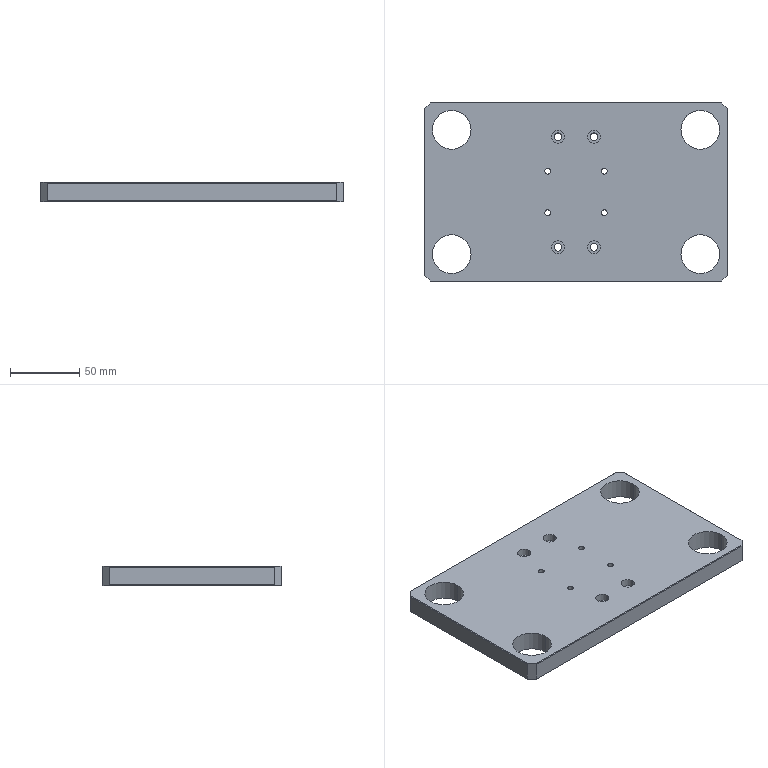Part | STEP file | Riveting slide mounting plate | 1 solid | 54 faces | box 220 x 130 x 14 mm | volume 361910 mm3 | cylinder 32 | plane 22 | commonest cylinder face diameters 4.2 x8 5.5 x8 9.5 x8 28 x8